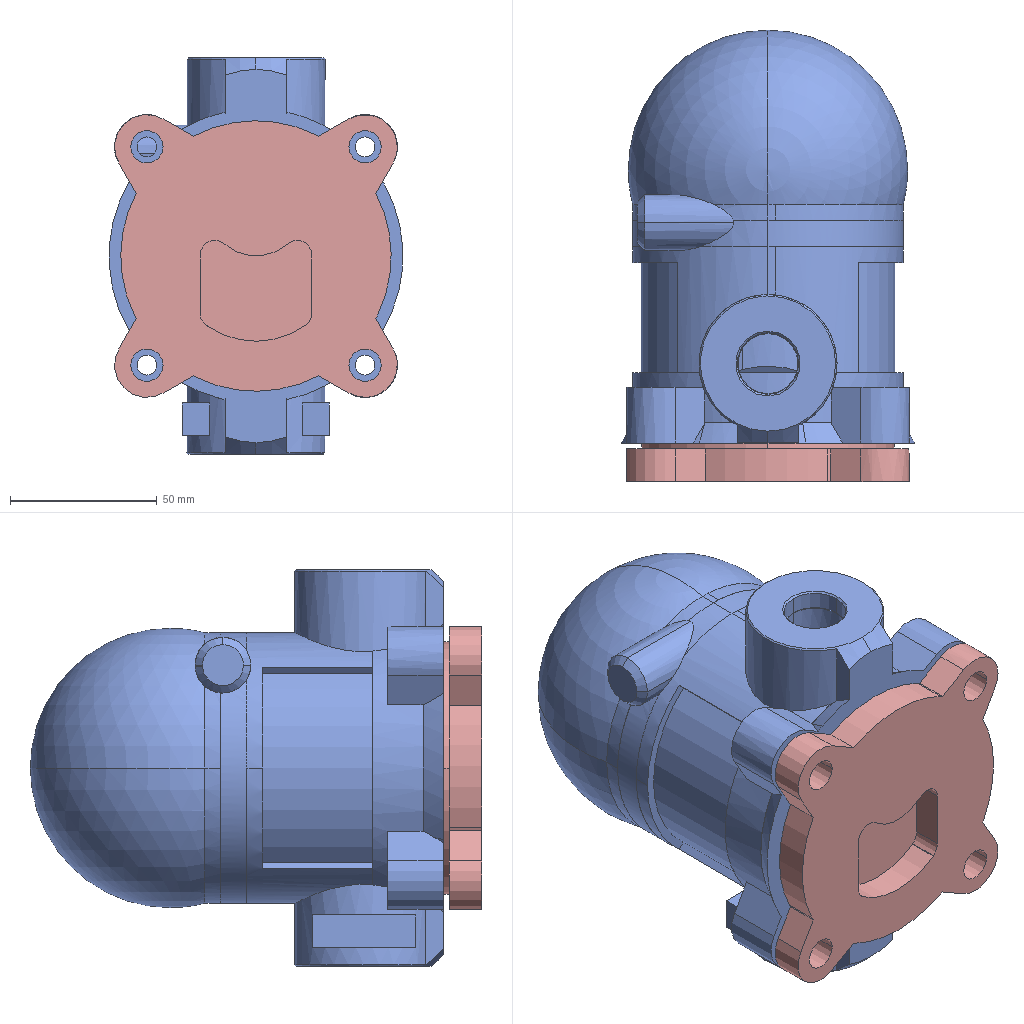Assembly | SolidWorks | 15 different items | 15 placed | box 100 x 154 x 135 mm
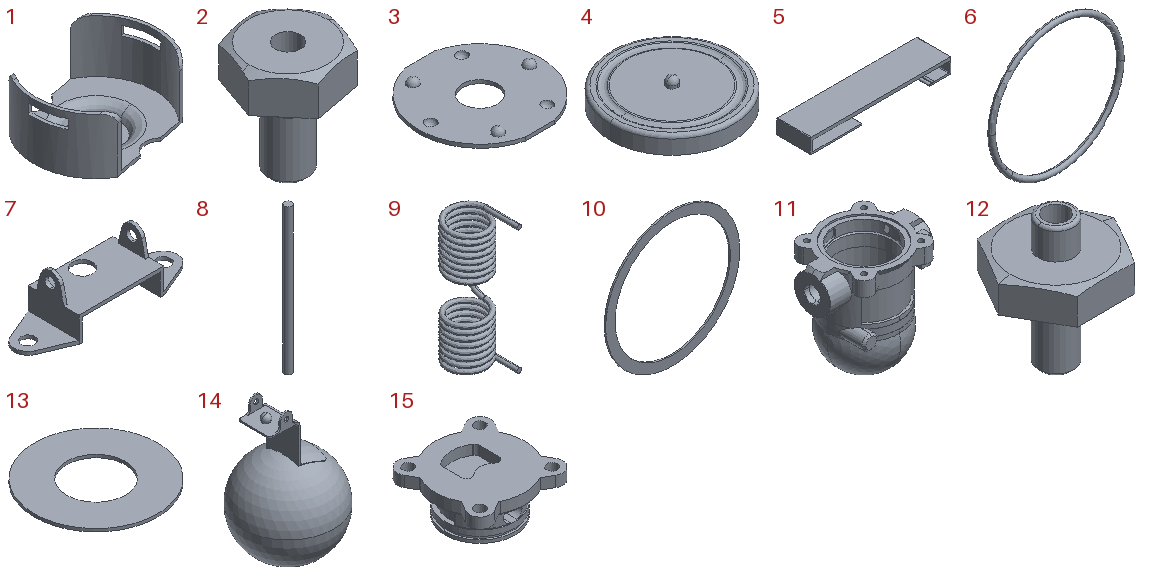Parts list (item | quantity | size | volume | features):
1 | x1 | 40 x 34.338 x 21 mm | 2143 mm3 | features Cut 4, Fillet 2, Extrusion 1, ICE 1, Shell 1
2 | x1 | 19.298 x 18.51 x 22 mm | 2117 mm3 | features Cut 1, Extrusion 1, Fillet 1, ICE 1, RevCut 1, StudWizard 1
3 | x1 | 35 x 34 x 4 mm | 890.444 mm3 | features CirPattern 4, RevCut 2, Revolution 2, Extrusion 1, ICE 1
4 | x1 | 35 x 35 x 10.3 mm | 4614 mm3 | features Fillet 2, RevCut 2, Revolution 2, Extrusion 1
5 | x1 | 42 x 10 x 4.5 mm | 558.172 mm3 | features ICE 4, Extrusion 1, Fillet 1
6 | x1 | 74 x 3 x 74 mm | 1577 mm3 | features Revolution 1
7 | x1 | 48 x 15 x 14.485 mm | 815.815 mm3 | features ICE 4, Cut 1, Extrusion 1
8 | x1 | 2.8 x 2.8 x 55 mm | 338.664 mm3 | features Extrusion 1
9 | x1 | 3.6 x 4.8 x 11.4 mm | 21.099 mm3 | features ICE 4, CompositeCurve 1, Helix 1, MirrorPattern 1, Scale 1, Sweep 1
10 | x1 | 86 x 1 x 86 mm | 1508 mm3 | features Extrusion 1
11 | x1 | 135 x 100 x 140.5 mm | 345567 mm3 | features ICE 9, Fillet 7, HoleWzd 2, Revolution 2, BaseBody 1, Chamfer 1, MirrorPattern 1, RevCut 1
12 | x1 | 19.63 x 17 x 22 mm | 1443 mm3 | features ICE 2, Cut 1, Extrusion 1, Fillet 1, RevCut 1, StudWizard 1
13 | x1 | 21 x 21 x 0.5 mm | 133.91 mm3 | features Extrusion 1
14 | x1 | 60 x 60 x 93.006 mm | 12285 mm3 | features Fillet 5, ICE 3, Revolution 3, MirrorPattern 1
15 | x1 | 96.247 x 96.248 x 43.6 mm | 156793 mm3 | features ICE 25, Fillet 7, HoleWzd 2, BaseBody 1
Mates (type | each side: item.copy, entity, surface, feature):
Coincident | 15.1 plane | assembly plane | 3 times
Concentric | 15.1 face cylinder Input1 | 11.1 face cylinder Input1 | 2 times
Concentric | 15.1 face cylinder Boss-Extrude4 | 11.1 face cylinder Cut-Extrude4
Concentric | 15.1 face cylinder Input1 | 10.1 face cylinder Boss-Extrude1
Coincident | 15.1 face plane Cut-Extrude2 | 10.1 face plane Boss-Extrude1
Coincident | 11.1 face plane Cut-Extrude2 | 10.1 face plane Boss-Extrude1
Coincident | 15.1 face plane Boss-Extrude10 | 13.1 face plane Boss-Extrude1
Concentric | 15.1 face cylinder Boss-Extrude10 | 13.1 face cylinder Boss-Extrude1
Concentric | 15.1 face cylinder Cut-Extrude17 | 1.1 face cylinder Cut-Extrude5
Parallel | 15.1 face plane Cut-Extrude14 | 1.1 face plane Cut-Extrude6
Coincident | 13.1 face plane Boss-Extrude1 | 1.1 face plane Boss-Extrude2
Concentric | 1.1 face cylinder Cut-Extrude5 | 2.1 face cylinder Boss-Extrude2
Coincident | 1.1 face plane Shell1 | 2.1 face plane Boss-Extrude1
Concentric | 2.1 face cylinder Cut-Extrude1 | 3.1 face cylinder Boss-Extrude1
Parallel | 1.1 face plane Cut-Extrude6 | 3.1 face plane Cut-Extrude1
Coincident | 2.1 face plane Boss-Extrude1 | 3.1 face plane Boss-Extrude1
Concentric | 1.1 face cylinder Shell1 | 4.1 face cylinder Boss-Extrude1
Coincident | 4.1 face plane Boss-Extrude1 | assembly plane
InPlace | 15.1 face plane Boss-Extrude12 | 7.1 plane
Coincident | 15.1 face plane Boss-Extrude13 | 12.1 face plane Boss-Extrude1
Concentric | 15.1 face cylinder M8 Tapped Hole1 | 12.1 face cylinder Boss-Extrude3
Perpendicular | 15.1 face plane Cut-Extrude14 | 12.1 face plane Boss-Extrude1
Parallel | 7.1 face plane Boss-Extrude3 | 14.1 face plane Boss-Extrude1
Parallel | 7.1 face plane Boss-Extrude2 | 14.1 face plane Boss-Extrude1
Width | 7.1 face plane Boss-Extrude2 | 7.1 face plane Boss-Extrude2 | 14.1 face plane Boss-Extrude1 | 14.1 face plane Boss-Extrude1
Concentric | 12.1 face cylinder Cut-Extrude1 | 14.1 face sphere Revolve3
Concentric | 7.1 face cylinder Boss-Extrude5 | 14.1 face cylinder Cut-Extrude1
InPlace | 5.1 plane | assembly plane
InPlace | 6.1 plane | assembly plane
Concentric | 7.1 face cylinder Boss-Extrude5 | 8.1 face cylinder Boss-Extrude1
Coincident | 8.1 axis | 9.1 select_type:24
Width | 8.1 face plane Boss-Extrude1 | 8.1 face plane Boss-Extrude1 | 7.1 face plane Boss-Extrude2 | 7.1 face plane Boss-Extrude2